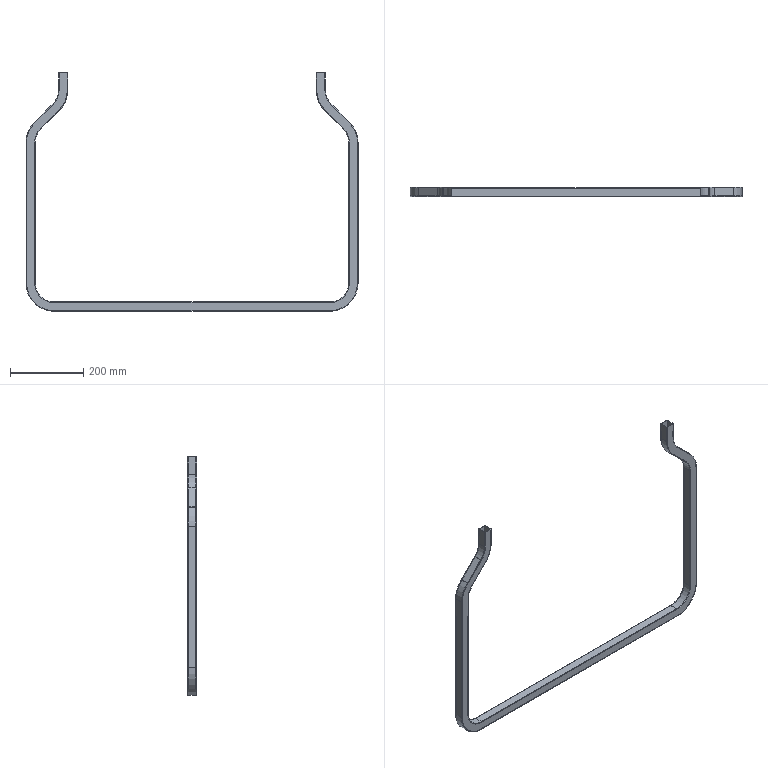Part | NX | features BREP 1 | 1 solid | 110 faces | box 908.05 x 25.4 x 652.272 mm | volume 379040 mm3 | cylinder 52 | plane 34 | torus 24 | commonest cylinder face diameters 3.175 x28 101.6 x6 105.359 x6 148.641 x6 152.4 x6